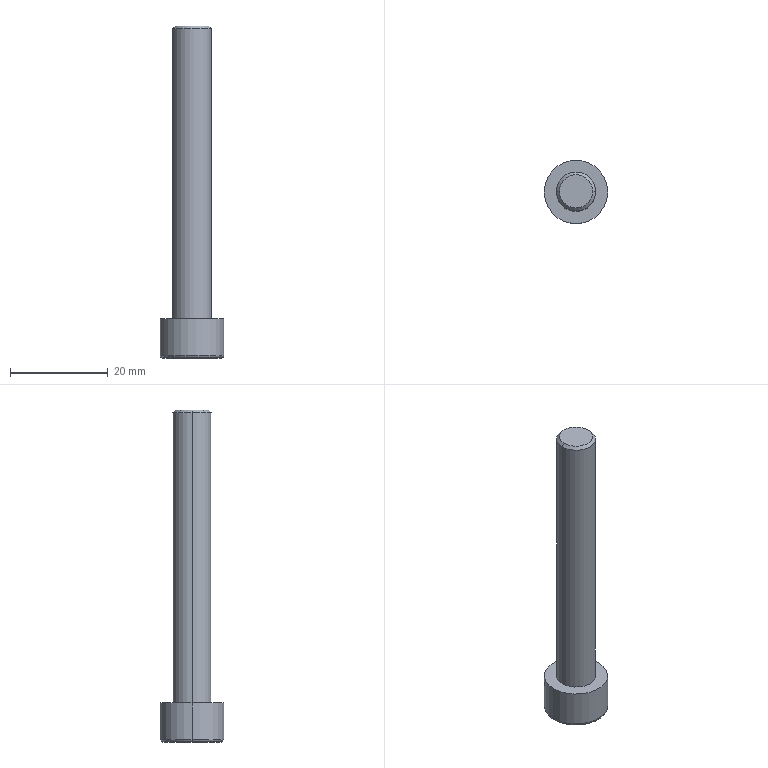Part | Creo | 1 solid | 20 faces | box 13 x 13 x 68 mm | volume 3907 mm3 | plane 10 | torus 4 | cylinder 4 | cone 2 | commonest cylinder face diameters 8 x2 13 x2
STEP:
#1=CARTESIAN_POINT('',(-39.,-355.,-43.5));
#2=VERTEX_POINT('',#1);
#3=CARTESIAN_POINT('',(-27.,-355.,-43.5));
#4=VERTEX_POINT('',#3);
#5=CARTESIAN_POINT('',(-33.,-355.,-43.5));
#6=DIRECTION('',(0.,0.,-1.));
#7=DIRECTION('',(-1.,0.,0.));
#8=AXIS2_PLACEMENT_3D('',#5,#6,#7);
#9=CIRCLE('',#8,6.);
#10=EDGE_CURVE('',#2,#4,#9,.T.);
#11=ORIENTED_EDGE('',*,*,#10,.F.);
#12=CARTESIAN_POINT('',(-33.,-355.,-43.5));
#13=DIRECTION('',(0.,0.,-1.));
#14=DIRECTION('',(1.,0.,0.));
#15=AXIS2_PLACEMENT_3D('',#12,#13,#14);
#16=CIRCLE('',#15,6.);
#17=EDGE_CURVE('',#4,#2,#16,.T.);
#18=ORIENTED_EDGE('',*,*,#17,.F.);
#19=EDGE_LOOP('',(#11,#18));
#20=FACE_OUTER_BOUND('',#19,.F.);
#21=CARTESIAN_POINT('',(-34.732,-352.,-43.5));
#22=VERTEX_POINT('',#21);
#23=CARTESIAN_POINT('',(-31.268,-352.,-43.5));
#24=VERTEX_POINT('',#23);
#25=CARTESIAN_POINT('',(-34.732,-352.,-43.5));
#26=DIRECTION('',(1.,0.,0.));
#27=VECTOR('',#26,3.464);
#28=LINE('',#25,#27);
#29=EDGE_CURVE('',#22,#24,#28,.T.);
#30=ORIENTED_EDGE('',*,*,#29,.T.);
#31=CARTESIAN_POINT('',(-29.536,-355.,-43.5));
#32=VERTEX_POINT('',#31);
#33=CARTESIAN_POINT('',(-29.536,-355.,-43.5));
#34=DIRECTION('',(-0.5,0.866,0.));
#35=VECTOR('',#34,3.464);
#36=LINE('',#33,#35);
#37=EDGE_CURVE('',#32,#24,#36,.T.);
#38=ORIENTED_EDGE('',*,*,#37,.F.);
#39=CARTESIAN_POINT('',(-31.268,-358.,-43.5));
#40=VERTEX_POINT('',#39);
#41=CARTESIAN_POINT('',(-31.268,-358.,-43.5));
#42=DIRECTION('',(0.5,0.866,0.));
#43=VECTOR('',#42,3.464);
#44=LINE('',#41,#43);
#45=EDGE_CURVE('',#40,#32,#44,.T.);
#46=ORIENTED_EDGE('',*,*,#45,.F.);
#47=CARTESIAN_POINT('',(-34.732,-358.,-43.5));
#48=VERTEX_POINT('',#47);
#49=CARTESIAN_POINT('',(-31.268,-358.,-43.5));
#50=DIRECTION('',(-1.,0.,0.));
#51=VECTOR('',#50,3.464);
#52=LINE('',#49,#51);
#53=EDGE_CURVE('',#40,#48,#52,.T.);
#54=ORIENTED_EDGE('',*,*,#53,.T.);
#55=CARTESIAN_POINT('',(-36.464,-355.,-43.5));
#56=VERTEX_POINT('',#55);
#57=CARTESIAN_POINT('',(-36.464,-355.,-43.5));
#58=DIRECTION('',(0.5,-0.866,0.));
#59=VECTOR('',#58,3.464);
#60=LINE('',#57,#59);
#61=EDGE_CURVE('',#56,#48,#60,.T.);
#62=ORIENTED_EDGE('',*,*,#61,.F.);
#63=CARTESIAN_POINT('',(-34.732,-352.,-43.5));
#64=DIRECTION('',(-0.5,-0.866,0.));
#65=VECTOR('',#64,3.464);
#66=LINE('',#63,#65);
#67=EDGE_CURVE('',#22,#56,#66,.T.);
#68=ORIENTED_EDGE('',*,*,#67,.F.);
#69=EDGE_LOOP('',(#30,#38,#46,#54,#62,#68));
#70=FACE_BOUND('',#69,.F.);
#71=CARTESIAN_POINT('',(-33.,-355.,-43.5));
#72=DIRECTION('',(0.,0.,-1.));
#73=DIRECTION('',(-1.,0.,0.));
#74=AXIS2_PLACEMENT_3D('',#71,#72,#73);
#75=PLANE('',#74);
#76=ADVANCED_FACE('',(#20,#70),#75,.T.);
#77=ORIENTED_EDGE('',*,*,#10,.T.);
#78=CARTESIAN_POINT('',(-26.646,-355.,-43.354));
#79=VERTEX_POINT('',#78);
#80=CARTESIAN_POINT('',(-27.,-355.,-43.));
#81=DIRECTION('',(0.,1.,0.));
#82=DIRECTION('',(0.7071,0.,-0.7071));
#83=AXIS2_PLACEMENT_3D('',#80,#81,#82);
#84=CIRCLE('',#83,0.5);
#85=EDGE_CURVE('',#79,#4,#84,.T.);
#86=ORIENTED_EDGE('',*,*,#85,.F.);
#87=CARTESIAN_POINT('',(-39.354,-355.,-43.354));
#88=VERTEX_POINT('',#87);
#89=CARTESIAN_POINT('',(-33.,-355.,-43.354));
#90=DIRECTION('',(0.,0.,-1.));
#91=DIRECTION('',(-1.,0.,0.));
#92=AXIS2_PLACEMENT_3D('',#89,#90,#91);
#93=CIRCLE('',#92,6.354);
#94=EDGE_CURVE('',#88,#79,#93,.T.);
#95=ORIENTED_EDGE('',*,*,#94,.F.);
#96=CARTESIAN_POINT('',(-39.,-355.,-43.));
#97=DIRECTION('',(0.,-1.,0.));
#98=DIRECTION('',(-0.7071,0.,-0.7071));
#99=AXIS2_PLACEMENT_3D('',#96,#97,#98);
#100=CIRCLE('',#99,0.5);
#101=EDGE_CURVE('',#88,#2,#100,.T.);
#102=ORIENTED_EDGE('',*,*,#101,.T.);
#103=EDGE_LOOP('',(#77,#86,#95,#102));
#104=FACE_OUTER_BOUND('',#103,.F.);
#105=CARTESIAN_POINT('',(-33.,-355.,-43.));
#106=DIRECTION('',(0.,0.,-1.));
#107=DIRECTION('',(-1.,0.,0.));
#108=AXIS2_PLACEMENT_3D('',#105,#106,#107);
#109=TOROIDAL_SURFACE('',#108,6.,0.5);
#110=ADVANCED_FACE('',(#104),#109,.T.);
#111=ORIENTED_EDGE('',*,*,#17,.T.);
#112=ORIENTED_EDGE('',*,*,#101,.F.);
#113=CARTESIAN_POINT('',(-33.,-355.,-43.354));
#114=DIRECTION('',(0.,0.,-1.));
#115=DIRECTION('',(1.,0.,0.));
#116=AXIS2_PLACEMENT_3D('',#113,#114,#115);
#117=CIRCLE('',#116,6.354);
#118=EDGE_CURVE('',#79,#88,#117,.T.);
#119=ORIENTED_EDGE('',*,*,#118,.F.);
#120=ORIENTED_EDGE('',*,*,#85,.T.);
#121=EDGE_LOOP('',(#111,#112,#119,#120));
#122=FACE_OUTER_BOUND('',#121,.F.);
#123=CARTESIAN_POINT('',(-33.,-355.,-43.));
#124=DIRECTION('',(0.,0.,-1.));
#125=DIRECTION('',(-1.,0.,0.));
#126=AXIS2_PLACEMENT_3D('',#123,#124,#125);
#127=TOROIDAL_SURFACE('',#126,6.,0.5);
#128=ADVANCED_FACE('',(#122),#127,.T.);
#129=CARTESIAN_POINT('',(-26.5,-355.,-43.));
#130=VERTEX_POINT('',#129);
#131=CARTESIAN_POINT('',(-39.5,-355.,-43.));
#132=VERTEX_POINT('',#131);
#133=CARTESIAN_POINT('',(-33.,-355.,-43.));
#134=DIRECTION('',(0.,0.,-1.));
#135=DIRECTION('',(1.,0.,0.));
#136=AXIS2_PLACEMENT_3D('',#133,#134,#135);
#137=CIRCLE('',#136,6.5);
#138=EDGE_CURVE('',#130,#132,#137,.T.);
#139=ORIENTED_EDGE('',*,*,#138,.F.);
#140=CARTESIAN_POINT('',(-27.,-355.,-43.));
#141=DIRECTION('',(0.,1.,0.));
#142=DIRECTION('',(1.,0.,0.));
#143=AXIS2_PLACEMENT_3D('',#140,#141,#142);
#144=CIRCLE('',#143,0.5);
#145=EDGE_CURVE('',#130,#79,#144,.T.);
#146=ORIENTED_EDGE('',*,*,#145,.T.);
#147=ORIENTED_EDGE('',*,*,#118,.T.);
#148=CARTESIAN_POINT('',(-39.,-355.,-43.));
#149=DIRECTION('',(0.,-1.,0.));
#150=DIRECTION('',(-1.,0.,0.));
#151=AXIS2_PLACEMENT_3D('',#148,#149,#150);
#152=CIRCLE('',#151,0.5);
#153=EDGE_CURVE('',#132,#88,#152,.T.);
#154=ORIENTED_EDGE('',*,*,#153,.F.);
#155=EDGE_LOOP('',(#139,#146,#147,#154));
#156=FACE_OUTER_BOUND('',#155,.F.);
#157=CARTESIAN_POINT('',(-33.,-355.,-43.));
#158=DIRECTION('',(0.,0.,-1.));
#159=DIRECTION('',(-1.,0.,0.));
#160=AXIS2_PLACEMENT_3D('',#157,#158,#159);
#161=TOROIDAL_SURFACE('',#160,6.,0.5);
#162=ADVANCED_FACE('',(#156),#161,.T.);
#163=ORIENTED_EDGE('',*,*,#138,.T.);
#164=CARTESIAN_POINT('',(-39.5,-355.,-35.5));
#165=VERTEX_POINT('',#164);
#166=CARTESIAN_POINT('',(-39.5,-355.,-35.5));
#167=DIRECTION('',(0.,0.,-1.));
#168=VECTOR('',#167,7.5);
#169=LINE('',#166,#168);
#170=EDGE_CURVE('',#165,#132,#169,.T.);
#171=ORIENTED_EDGE('',*,*,#170,.F.);
#172=CARTESIAN_POINT('',(-26.5,-355.,-35.5));
#173=VERTEX_POINT('',#172);
#174=CARTESIAN_POINT('',(-33.,-355.,-35.5));
#175=DIRECTION('',(0.,0.,1.));
#176=DIRECTION('',(-1.,0.,0.));
#177=AXIS2_PLACEMENT_3D('',#174,#175,#176);
#178=CIRCLE('',#177,6.5);
#179=EDGE_CURVE('',#165,#173,#178,.T.);
#180=ORIENTED_EDGE('',*,*,#179,.T.);
#181=CARTESIAN_POINT('',(-26.5,-355.,-35.5));
#182=DIRECTION('',(0.,0.,-1.));
#183=VECTOR('',#182,7.5);
#184=LINE('',#181,#183);
#185=EDGE_CURVE('',#173,#130,#184,.T.);
#186=ORIENTED_EDGE('',*,*,#185,.T.);
#187=EDGE_LOOP('',(#163,#171,#180,#186));
#188=FACE_OUTER_BOUND('',#187,.F.);
#189=CARTESIAN_POINT('',(-33.,-355.,-35.5));
#190=DIRECTION('',(0.,0.,-1.));
#191=DIRECTION('',(-1.,0.,0.));
#192=AXIS2_PLACEMENT_3D('',#189,#190,#191);
#193=CYLINDRICAL_SURFACE('',#192,6.5);
#194=ADVANCED_FACE('',(#188),#193,.T.);
#195=CARTESIAN_POINT('',(-33.,-355.,-43.));
#196=DIRECTION('',(0.,0.,-1.));
#197=DIRECTION('',(-1.,0.,0.));
#198=AXIS2_PLACEMENT_3D('',#195,#196,#197);
#199=CIRCLE('',#198,6.5);
#200=EDGE_CURVE('',#132,#130,#199,.T.);
#201=ORIENTED_EDGE('',*,*,#200,.T.);
#202=ORIENTED_EDGE('',*,*,#185,.F.);
#203=CARTESIAN_POINT('',(-33.,-355.,-35.5));
#204=DIRECTION('',(0.,0.,1.));
#205=DIRECTION('',(1.,0.,0.));
#206=AXIS2_PLACEMENT_3D('',#203,#204,#205);
#207=CIRCLE('',#206,6.5);
#208=EDGE_CURVE('',#173,#165,#207,.T.);
#209=ORIENTED_EDGE('',*,*,#208,.T.);
#210=ORIENTED_EDGE('',*,*,#170,.T.);
#211=EDGE_LOOP('',(#201,#202,#209,#210));
#212=FACE_OUTER_BOUND('',#211,.F.);
#213=CARTESIAN_POINT('',(-33.,-355.,-35.5));
#214=DIRECTION('',(0.,0.,-1.));
#215=DIRECTION('',(-1.,0.,0.));
#216=AXIS2_PLACEMENT_3D('',#213,#214,#215);
#217=CYLINDRICAL_SURFACE('',#216,6.5);
#218=ADVANCED_FACE('',(#212),#217,.T.);
#219=ORIENTED_EDGE('',*,*,#200,.F.);
#220=ORIENTED_EDGE('',*,*,#153,.T.);
#221=ORIENTED_EDGE('',*,*,#94,.T.);
#222=ORIENTED_EDGE('',*,*,#145,.F.);
#223=EDGE_LOOP('',(#219,#220,#221,#222));
#224=FACE_OUTER_BOUND('',#223,.F.);
#225=CARTESIAN_POINT('',(-33.,-355.,-43.));
#226=DIRECTION('',(0.,0.,-1.));
#227=DIRECTION('',(-1.,0.,0.));
#228=AXIS2_PLACEMENT_3D('',#225,#226,#227);
#229=TOROIDAL_SURFACE('',#228,6.,0.5);
#230=ADVANCED_FACE('',(#224),#229,.T.);
#231=ORIENTED_EDGE('',*,*,#179,.F.);
#232=ORIENTED_EDGE('',*,*,#208,.F.);
#233=EDGE_LOOP('',(#231,#232));
#234=FACE_OUTER_BOUND('',#233,.F.);
#235=CARTESIAN_POINT('',(-37.,-355.,-35.5));
#236=VERTEX_POINT('',#235);
#237=CARTESIAN_POINT('',(-29.,-355.,-35.5));
#238=VERTEX_POINT('',#237);
#239=CARTESIAN_POINT('',(-33.,-355.,-35.5));
#240=DIRECTION('',(0.,0.,-1.));
#241=DIRECTION('',(-1.,0.,0.));
#242=AXIS2_PLACEMENT_3D('',#239,#240,#241);
#243=CIRCLE('',#242,4.);
#244=EDGE_CURVE('',#236,#238,#243,.T.);
#245=ORIENTED_EDGE('',*,*,#244,.F.);
#246=CARTESIAN_POINT('',(-33.,-355.,-35.5));
#247=DIRECTION('',(0.,0.,-1.));
#248=DIRECTION('',(1.,0.,0.));
#249=AXIS2_PLACEMENT_3D('',#246,#247,#248);
#250=CIRCLE('',#249,4.);
#251=EDGE_CURVE('',#238,#236,#250,.T.);
#252=ORIENTED_EDGE('',*,*,#251,.F.);
#253=EDGE_LOOP('',(#245,#252));
#254=FACE_BOUND('',#253,.F.);
#255=CARTESIAN_POINT('',(-33.,-355.,-35.5));
#256=DIRECTION('',(0.,0.,1.));
#257=DIRECTION('',(1.,0.,0.));
#258=AXIS2_PLACEMENT_3D('',#255,#256,#257);
#259=PLANE('',#258);
#260=ADVANCED_FACE('',(#234,#254),#259,.T.);
#261=CARTESIAN_POINT('',(-29.,-355.,23.9));
#262=VERTEX_POINT('',#261);
#263=CARTESIAN_POINT('',(-37.,-355.,23.9));
#264=VERTEX_POINT('',#263);
#265=CARTESIAN_POINT('',(-33.,-355.,23.9));
#266=DIRECTION('',(0.,0.,1.));
#267=DIRECTION('',(1.,0.,0.));
#268=AXIS2_PLACEMENT_3D('',#265,#266,#267);
#269=CIRCLE('',#268,4.);
#270=EDGE_CURVE('',#262,#264,#269,.T.);
#271=ORIENTED_EDGE('',*,*,#270,.T.);
#272=CARTESIAN_POINT('',(-37.,-355.,23.9));
#273=DIRECTION('',(0.,0.,-1.));
#274=VECTOR('',#273,59.4);
#275=LINE('',#272,#274);
#276=EDGE_CURVE('',#264,#236,#275,.T.);
#277=ORIENTED_EDGE('',*,*,#276,.T.);
#278=ORIENTED_EDGE('',*,*,#244,.T.);
#279=CARTESIAN_POINT('',(-29.,-355.,23.9));
#280=DIRECTION('',(0.,0.,-1.));
#281=VECTOR('',#280,59.4);
#282=LINE('',#279,#281);
#283=EDGE_CURVE('',#262,#238,#282,.T.);
#284=ORIENTED_EDGE('',*,*,#283,.F.);
#285=EDGE_LOOP('',(#271,#277,#278,#284));
#286=FACE_OUTER_BOUND('',#285,.F.);
#287=CARTESIAN_POINT('',(-33.,-355.,24.5));
#288=DIRECTION('',(0.,0.,-1.));
#289=DIRECTION('',(-1.,0.,0.));
#290=AXIS2_PLACEMENT_3D('',#287,#288,#289);
#291=CYLINDRICAL_SURFACE('',#290,4.);
#292=ADVANCED_FACE('',(#286),#291,.T.);
#293=CARTESIAN_POINT('',(-29.6,-355.,24.5));
#294=VERTEX_POINT('',#293);
#295=CARTESIAN_POINT('',(-36.4,-355.,24.5));
#296=VERTEX_POINT('',#295);
#297=CARTESIAN_POINT('',(-33.,-355.,24.5));
#298=DIRECTION('',(0.,0.,1.));
#299=DIRECTION('',(1.,0.,0.));
#300=AXIS2_PLACEMENT_3D('',#297,#298,#299);
#301=CIRCLE('',#300,3.4);
#302=EDGE_CURVE('',#294,#296,#301,.T.);
#303=ORIENTED_EDGE('',*,*,#302,.T.);
#304=CARTESIAN_POINT('',(-36.4,-355.,24.5));
#305=DIRECTION('',(-0.7071,0.,-0.7071));
#306=VECTOR('',#305,0.8485);
#307=LINE('',#304,#306);
#308=EDGE_CURVE('',#296,#264,#307,.T.);
#309=ORIENTED_EDGE('',*,*,#308,.T.);
#310=ORIENTED_EDGE('',*,*,#270,.F.);
#311=CARTESIAN_POINT('',(-29.6,-355.,24.5));
#312=DIRECTION('',(0.7071,0.,-0.7071));
#313=VECTOR('',#312,0.8485);
#314=LINE('',#311,#313);
#315=EDGE_CURVE('',#294,#262,#314,.T.);
#316=ORIENTED_EDGE('',*,*,#315,.F.);
#317=EDGE_LOOP('',(#303,#309,#310,#316));
#318=FACE_OUTER_BOUND('',#317,.F.);
#319=CARTESIAN_POINT('',(-33.,-355.,24.2));
#320=DIRECTION('',(0.,0.,-1.));
#321=DIRECTION('',(-1.,0.,0.));
#322=AXIS2_PLACEMENT_3D('',#319,#320,#321);
#323=CONICAL_SURFACE('',#322,3.7,45.);
#324=ADVANCED_FACE('',(#318),#323,.T.);
#325=CARTESIAN_POINT('',(-33.,-355.,24.5));
#326=DIRECTION('',(0.,0.,1.));
#327=DIRECTION('',(-1.,0.,0.));
#328=AXIS2_PLACEMENT_3D('',#325,#326,#327);
#329=CIRCLE('',#328,3.4);
#330=EDGE_CURVE('',#296,#294,#329,.T.);
#331=ORIENTED_EDGE('',*,*,#330,.F.);
#332=ORIENTED_EDGE('',*,*,#302,.F.);
#333=EDGE_LOOP('',(#331,#332));
#334=FACE_OUTER_BOUND('',#333,.F.);
#335=CARTESIAN_POINT('',(-33.,-355.,24.5));
#336=DIRECTION('',(0.,0.,-1.));
#337=DIRECTION('',(-1.,0.,0.));
#338=AXIS2_PLACEMENT_3D('',#335,#336,#337);
#339=PLANE('',#338);
#340=ADVANCED_FACE('',(#334),#339,.F.);
#341=ORIENTED_EDGE('',*,*,#330,.T.);
#342=ORIENTED_EDGE('',*,*,#315,.T.);
#343=CARTESIAN_POINT('',(-33.,-355.,23.9));
#344=DIRECTION('',(0.,0.,1.));
#345=DIRECTION('',(-1.,0.,0.));
#346=AXIS2_PLACEMENT_3D('',#343,#344,#345);
#347=CIRCLE('',#346,4.);
#348=EDGE_CURVE('',#264,#262,#347,.T.);
#349=ORIENTED_EDGE('',*,*,#348,.F.);
#350=ORIENTED_EDGE('',*,*,#308,.F.);
#351=EDGE_LOOP('',(#341,#342,#349,#350));
#352=FACE_OUTER_BOUND('',#351,.F.);
#353=CARTESIAN_POINT('',(-33.,-355.,24.2));
#354=DIRECTION('',(0.,0.,-1.));
#355=DIRECTION('',(-1.,0.,0.));
#356=AXIS2_PLACEMENT_3D('',#353,#354,#355);
#357=CONICAL_SURFACE('',#356,3.7,45.);
#358=ADVANCED_FACE('',(#352),#357,.T.);
#359=ORIENTED_EDGE('',*,*,#348,.T.);
#360=ORIENTED_EDGE('',*,*,#283,.T.);
#361=ORIENTED_EDGE('',*,*,#251,.T.);
#362=ORIENTED_EDGE('',*,*,#276,.F.);
#363=EDGE_LOOP('',(#359,#360,#361,#362));
#364=FACE_OUTER_BOUND('',#363,.F.);
#365=CARTESIAN_POINT('',(-33.,-355.,24.5));
#366=DIRECTION('',(0.,0.,-1.));
#367=DIRECTION('',(-1.,0.,0.));
#368=AXIS2_PLACEMENT_3D('',#365,#366,#367);
#369=CYLINDRICAL_SURFACE('',#368,4.);
#370=ADVANCED_FACE('',(#364),#369,.T.);
#371=ORIENTED_EDGE('',*,*,#29,.F.);
#372=CARTESIAN_POINT('',(-34.732,-352.,-38.22));
#373=VERTEX_POINT('',#372);
#374=CARTESIAN_POINT('',(-34.732,-352.,-43.5));
#375=DIRECTION('',(0.,0.,1.));
#376=VECTOR('',#375,5.28);
#377=LINE('',#374,#376);
#378=EDGE_CURVE('',#22,#373,#377,.T.);
#379=ORIENTED_EDGE('',*,*,#378,.T.);
#380=CARTESIAN_POINT('',(-31.268,-352.,-38.22));
#381=VERTEX_POINT('',#380);
#382=CARTESIAN_POINT('',(-34.732,-352.,-38.22));
#383=DIRECTION('',(1.,0.,0.));
#384=VECTOR('',#383,3.464);
#385=LINE('',#382,#384);
#386=EDGE_CURVE('',#373,#381,#385,.T.);
#387=ORIENTED_EDGE('',*,*,#386,.T.);
#388=CARTESIAN_POINT('',(-31.268,-352.,-43.5));
#389=DIRECTION('',(0.,0.,1.));
#390=VECTOR('',#389,5.28);
#391=LINE('',#388,#390);
#392=EDGE_CURVE('',#24,#381,#391,.T.);
#393=ORIENTED_EDGE('',*,*,#392,.F.);
#394=EDGE_LOOP('',(#371,#379,#387,#393));
#395=FACE_OUTER_BOUND('',#394,.F.);
#396=CARTESIAN_POINT('',(-31.268,-352.,-38.22));
#397=DIRECTION('',(0.,-1.,0.));
#398=DIRECTION('',(0.,0.,1.));
#399=AXIS2_PLACEMENT_3D('',#396,#397,#398);
#400=PLANE('',#399);
#401=ADVANCED_FACE('',(#395),#400,.T.);
#402=ORIENTED_EDGE('',*,*,#67,.T.);
#403=CARTESIAN_POINT('',(-36.464,-355.,-38.22));
#404=VERTEX_POINT('',#403);
#405=CARTESIAN_POINT('',(-36.464,-355.,-43.5));
#406=DIRECTION('',(0.,0.,1.));
#407=VECTOR('',#406,5.28);
#408=LINE('',#405,#407);
#409=EDGE_CURVE('',#56,#404,#408,.T.);
#410=ORIENTED_EDGE('',*,*,#409,.T.);
#411=CARTESIAN_POINT('',(-36.464,-355.,-38.22));
#412=DIRECTION('',(0.5,0.866,0.));
#413=VECTOR('',#412,3.464);
#414=LINE('',#411,#413);
#415=EDGE_CURVE('',#404,#373,#414,.T.);
#416=ORIENTED_EDGE('',*,*,#415,.T.);
#417=ORIENTED_EDGE('',*,*,#378,.F.);
#418=EDGE_LOOP('',(#402,#410,#416,#417));
#419=FACE_OUTER_BOUND('',#418,.F.);
#420=CARTESIAN_POINT('',(-34.732,-352.,-38.22));
#421=DIRECTION('',(0.866,-0.5,0.));
#422=DIRECTION('',(-0.5,-0.866,0.));
#423=AXIS2_PLACEMENT_3D('',#420,#421,#422);
#424=PLANE('',#423);
#425=ADVANCED_FACE('',(#419),#424,.T.);
#426=ORIENTED_EDGE('',*,*,#61,.T.);
#427=CARTESIAN_POINT('',(-34.732,-358.,-38.22));
#428=VERTEX_POINT('',#427);
#429=CARTESIAN_POINT('',(-34.732,-358.,-43.5));
#430=DIRECTION('',(0.,0.,1.));
#431=VECTOR('',#430,5.28);
#432=LINE('',#429,#431);
#433=EDGE_CURVE('',#48,#428,#432,.T.);
#434=ORIENTED_EDGE('',*,*,#433,.T.);
#435=CARTESIAN_POINT('',(-34.732,-358.,-38.22));
#436=DIRECTION('',(-0.5,0.866,0.));
#437=VECTOR('',#436,3.464);
#438=LINE('',#435,#437);
#439=EDGE_CURVE('',#428,#404,#438,.T.);
#440=ORIENTED_EDGE('',*,*,#439,.T.);
#441=ORIENTED_EDGE('',*,*,#409,.F.);
#442=EDGE_LOOP('',(#426,#434,#440,#441));
#443=FACE_OUTER_BOUND('',#442,.F.);
#444=CARTESIAN_POINT('',(-36.464,-355.,-38.22));
#445=DIRECTION('',(0.866,0.5,0.));
#446=DIRECTION('',(0.5,-0.866,0.));
#447=AXIS2_PLACEMENT_3D('',#444,#445,#446);
#448=PLANE('',#447);
#449=ADVANCED_FACE('',(#443),#448,.T.);
#450=ORIENTED_EDGE('',*,*,#53,.F.);
#451=CARTESIAN_POINT('',(-31.268,-358.,-38.22));
#452=VERTEX_POINT('',#451);
#453=CARTESIAN_POINT('',(-31.268,-358.,-43.5));
#454=DIRECTION('',(0.,0.,1.));
#455=VECTOR('',#454,5.28);
#456=LINE('',#453,#455);
#457=EDGE_CURVE('',#40,#452,#456,.T.);
#458=ORIENTED_EDGE('',*,*,#457,.T.);
#459=CARTESIAN_POINT('',(-31.268,-358.,-38.22));
#460=DIRECTION('',(-1.,0.,0.));
#461=VECTOR('',#460,3.464);
#462=LINE('',#459,#461);
#463=EDGE_CURVE('',#452,#428,#462,.T.);
#464=ORIENTED_EDGE('',*,*,#463,.T.);
#465=ORIENTED_EDGE('',*,*,#433,.F.);
#466=EDGE_LOOP('',(#450,#458,#464,#465));
#467=FACE_OUTER_BOUND('',#466,.F.);
#468=CARTESIAN_POINT('',(-34.732,-358.,-38.22));
#469=DIRECTION('',(0.,1.,0.));
#470=DIRECTION('',(0.,0.,-1.));
#471=AXIS2_PLACEMENT_3D('',#468,#469,#470);
#472=PLANE('',#471);
#473=ADVANCED_FACE('',(#467),#472,.T.);
#474=ORIENTED_EDGE('',*,*,#45,.T.);
#475=CARTESIAN_POINT('',(-29.536,-355.,-38.22));
#476=VERTEX_POINT('',#475);
#477=CARTESIAN_POINT('',(-29.536,-355.,-43.5));
#478=DIRECTION('',(0.,0.,1.));
#479=VECTOR('',#478,5.28);
#480=LINE('',#477,#479);
#481=EDGE_CURVE('',#32,#476,#480,.T.);
#482=ORIENTED_EDGE('',*,*,#481,.T.);
#483=CARTESIAN_POINT('',(-29.536,-355.,-38.22));
#484=DIRECTION('',(-0.5,-0.866,0.));
#485=VECTOR('',#484,3.464);
#486=LINE('',#483,#485);
#487=EDGE_CURVE('',#476,#452,#486,.T.);
#488=ORIENTED_EDGE('',*,*,#487,.T.);
#489=ORIENTED_EDGE('',*,*,#457,.F.);
#490=EDGE_LOOP('',(#474,#482,#488,#489));
#491=FACE_OUTER_BOUND('',#490,.F.);
#492=CARTESIAN_POINT('',(-31.268,-358.,-38.22));
#493=DIRECTION('',(-0.866,0.5,0.));
#494=DIRECTION('',(0.5,0.866,0.));
#495=AXIS2_PLACEMENT_3D('',#492,#493,#494);
#496=PLANE('',#495);
#497=ADVANCED_FACE('',(#491),#496,.T.);
#498=ORIENTED_EDGE('',*,*,#37,.T.);
#499=ORIENTED_EDGE('',*,*,#392,.T.);
#500=CARTESIAN_POINT('',(-31.268,-352.,-38.22));
#501=DIRECTION('',(0.5,-0.866,0.));
#502=VECTOR('',#501,3.464);
#503=LINE('',#500,#502);
#504=EDGE_CURVE('',#381,#476,#503,.T.);
#505=ORIENTED_EDGE('',*,*,#504,.T.);
#506=ORIENTED_EDGE('',*,*,#481,.F.);
#507=EDGE_LOOP('',(#498,#499,#505,#506));
#508=FACE_OUTER_BOUND('',#507,.F.);
#509=CARTESIAN_POINT('',(-29.536,-355.,-38.22));
#510=DIRECTION('',(-0.866,-0.5,0.));
#511=DIRECTION('',(-0.5,0.866,0.));
#512=AXIS2_PLACEMENT_3D('',#509,#510,#511);
#513=PLANE('',#512);
#514=ADVANCED_FACE('',(#508),#513,.T.);
#515=ORIENTED_EDGE('',*,*,#415,.F.);
#516=ORIENTED_EDGE('',*,*,#439,.F.);
#517=ORIENTED_EDGE('',*,*,#463,.F.);
#518=ORIENTED_EDGE('',*,*,#487,.F.);
#519=ORIENTED_EDGE('',*,*,#504,.F.);
#520=ORIENTED_EDGE('',*,*,#386,.F.);
#521=EDGE_LOOP('',(#515,#516,#517,#518,#519,#520));
#522=FACE_OUTER_BOUND('',#521,.F.);
#523=CARTESIAN_POINT('',(-38.196,-358.,-38.22));
#524=DIRECTION('',(0.,0.,1.));
#525=DIRECTION('',(1.,0.,0.));
#526=AXIS2_PLACEMENT_3D('',#523,#524,#525);
#527=PLANE('',#526);
#528=ADVANCED_FACE('',(#522),#527,.F.);
#529=CLOSED_SHELL('',(#76,#110,#128,#162,#194,#218,#230,#260,#292,#324,#340,#358,#370,#401,#425,#449,#473,#497,#514,#528));
#530=MANIFOLD_SOLID_BREP('',#529);
#531=(LENGTH_UNIT()NAMED_UNIT(*)SI_UNIT(.MILLI.,.METRE.));
#532=UNCERTAINTY_MEASURE_WITH_UNIT(LENGTH_MEASURE(0.007044),#531,'','');
#533=(NAMED_UNIT(*)PLANE_ANGLE_UNIT()SI_UNIT($,.RADIAN.));
#534=PLANE_ANGLE_MEASURE_WITH_UNIT(PLANE_ANGLE_MEASURE(0.01745),#533);
#535=(CONVERSION_BASED_UNIT('DEGREE',#534)NAMED_UNIT(*)PLANE_ANGLE_UNIT());
#536=(NAMED_UNIT(*)SI_UNIT($,.STERADIAN.)SOLID_ANGLE_UNIT());
#537=(GEOMETRIC_REPRESENTATION_CONTEXT(3)GLOBAL_UNCERTAINTY_ASSIGNED_CONTEXT((#532))GLOBAL_UNIT_ASSIGNED_CONTEXT((#531,#535,#536))REPRESENTATION_CONTEXT('',''));
#538=ADVANCED_BREP_SHAPE_REPRESENTATION('',(#530),#537);